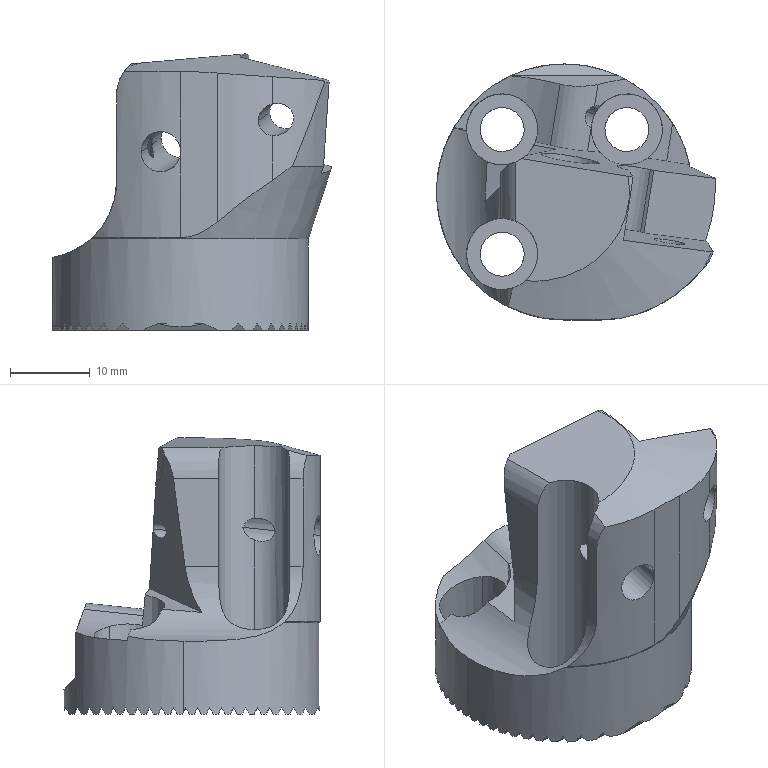NC program | Mastercam | posted with a generic post
Lines 6703 to 7888 of 7888:
(12 FEMR |TOOL - 4|DIA. OFF. - 4|LEN. - 4|TOOL DIA. - 12.)
N3534 T4 M6
N3536 G0 G54 G90 X-14.045 Y10.129 C-102.311 B-16.13 S3500 M3
N3538 G43 H4 Z65.102
N3540 Z17.102
N3542 G1 Z15.352 F2000.
N3544 X-12.727 Y9.028 Z15.201
N3546 G3 X-11.738 Y8.504 Z15.102 I1.732 J2.072
N3548 G1 X-11.151 Y8.336
N3550 X-11.015 Y8.564
N3552 G3 X-10.442 Y10.028 I-12.999 J5.944
N3554 G2 X-7.242 Y13.686 I6.178 J-2.175
N3556 X-3.552 Y14.596 I3.801 J-7.478
N3558 X-.802 Y14.328 I.15 J-12.665
N3560 X-.481 Y14.256 I-2.599 J-12.397
N3562 X1.84 Y13.588 I-5.294 J-22.736
N3564 G1 X1.993 Y13.964
N3566 X2.147 Y14.341
N3568 G3 X2.287 Y14.803 Z15.134 I-2.502 J1.016
N3570 X1.079 Y17.644 Z15.352 I-2.643 J.554
N3572 X.198 Y17.999 I-1.435 J-2.287
N3574 X-1.363 Y17.862 I-.554 J-2.643
N3576 G1 X-11.97 Y13.595 F9500.
N3578 G3 X-13.605 Y11.644 I1.007 J-2.505
N3580 X-13.648 Y11.37 I2.643 J-.554
N3582 X-11.704 Y8.494 Z15.102 I2.686 J-.28 F2000.
N3584 G1 X-11.118 Y8.327
N3586 X-11.094 Y8.32
N3588 G3 X-10.684 Y8.999 I-2.593 J2.03
N3590 G2 X-5.541 Y13.373 I7.474 J-3.577
N3592 X-1.371 Y13.742 I3.019 J-10.401
N3594 X.451 Y13.496 I-4.751 J-42.131
N3596 X1.721 Y13.293 I-1.718 J-14.847
N3598 G1 X1.874 Y13.67
N3600 X2.027 Y14.047
N3602 G3 X2.168 Y14.509 Z15.134 I-2.502 J1.016
N3604 X.96 Y17.35 Z15.352 I-2.643 J.554
N3606 X.08 Y17.705 I-1.435 J-2.287 F9500.
N3608 X-1.44 Y17.585 I-.554 J-2.643
N3610 G1 X-11.864 Y13.594
N3612 G3 X-13.542 Y11.626 I.965 J-2.522
N3614 X-13.584 Y11.352 I2.643 J-.554
N3616 X-11.641 Y8.476 Z15.102 I2.685 J-.28 F2000.
N3618 G1 X-11.054 Y8.308
N3620 X-11.022 Y8.299
N3622 G3 X-10.735 Y8.651 I-1.313 J1.369
N3624 G2 X-8.574 Y10.989 I9.204 J-6.338
N3626 X-3.748 Y13.028 I6.128 J-7.774
N3628 X-.057 Y13.105 I2.194 J-16.712
N3630 G3 X1.169 Y13.049 I2.21 J34.681
N3632 G2 X1.606 Y13.011 I-.779 J-11.644
N3634 G1 X1.759 Y13.388
N3636 X1.913 Y13.765
N3638 G3 X2.053 Y14.227 Z15.134 I-2.501 J1.016
N3640 X.846 Y17.068 Z15.352 I-2.642 J.554
N3642 X-.035 Y17.423 I-1.435 J-2.286 F9500.
N3644 X-1.515 Y17.317 I-.554 J-2.642
N3646 G1 X-11.737 Y13.583
N3648 G3 X-13.453 Y11.601 I.927 J-2.536
N3650 X-13.496 Y11.327 I2.643 J-.554
N3652 X-11.553 Y8.451 Z15.102 I2.686 J-.28 F2000.
N3654 G1 X-10.966 Y8.283
N3656 X-10.911 Y8.268
N3658 G3 X-10.36 Y8.798 I-2.825 J3.488
N3660 G2 X-7.106 Y11.303 I8.864 J-8.152
N3662 X-2.798 Y12.561 I5.527 J-10.906
N3664 X.131 Y12.699 I2.704 J-26.227
N3666 G3 X.733 Y12.722 I-.134 J11.466
N3668 G2 X1.494 Y12.735 I.545 J-10.028
N3670 G1 X1.647 Y13.112
N3672 X1.801 Y13.489
N3674 G3 X1.941 Y13.952 Z15.134 I-2.501 J1.016
N3676 X.734 Y16.793 Z15.352 I-2.642 J.554
N3678 X-.147 Y17.148 I-1.435 J-2.287 F9500.
N3680 X-1.597 Y17.053 I-.554 J-2.643
N3682 G1 X-11.552 Y13.55
N3684 G3 X-13.298 Y11.556 I.896 J-2.547
N3686 X-13.341 Y11.282 I2.643 J-.554
N3688 X-11.398 Y8.406 Z15.102 I2.686 J-.28 F2000.
N3690 G1 X-10.81 Y8.239
N3692 X-10.731 Y8.216
N3694 G3 X-10.082 Y8.726 I-2.872 J4.324
N3696 G2 X-6.668 Y10.949 I9.276 J-10.51
N3698 X-2.761 Y12.063 I5.886 J-13.243
N3700 X.33 Y12.36 I5.444 J-40.371
N3702 X1.387 Y12.471 I2.596 J-19.798
N3704 G1 X1.54 Y12.847
N3706 X1.693 Y13.225
N3708 G3 X1.835 Y13.687 Z15.134 I-2.502 J1.016
N3710 X.626 Y16.527 Z15.352 I-2.643 J.554
N3712 X-.254 Y16.883 I-1.435 J-2.286 F9500.
N3714 X-1.681 Y16.795 I-.554 J-2.642
N3716 G1 X-11.329 Y13.501
N3718 G3 X-13.099 Y11.499 I.872 J-2.555
N3720 X-13.142 Y11.225 I2.643 J-.554
N3722 X-11.199 Y8.35 Z15.102 I2.686 J-.28 F2000.
N3724 G1 X-10.612 Y8.182
N3726 X-10.515 Y8.155
N3728 G3 X-9.836 Y8.598 I-2.432 J4.464
N3730 G2 X-6.087 Y10.689 I10.05 J-13.614
N3732 X-1.813 Y11.757 I6.66 J-17.566
N3734 X.191 Y12.025 I17.327 J-122.508
N3736 G3 X.868 Y12.143 I-2.05 J13.62
N3738 G1 X1.278 Y12.202
N3740 X1.584 Y12.956
N3742 G3 X1.725 Y13.419 Z15.134 I-2.502 J1.016
N3744 X.517 Y16.26 Z15.352 I-2.643 J.554
N3746 X-.364 Y16.615 I-1.435 J-2.287 F9500.
N3748 X-1.768 Y16.535 I-.554 J-2.643
N3750 G1 X-11.083 Y13.444
N3752 G3 X-12.874 Y11.436 I.85 J-2.562
N3754 X-12.918 Y11.161 I2.642 J-.554
N3756 X-10.974 Y8.286 Z15.102 I2.686 J-.279 F2000.
N3758 G1 X-10.387 Y8.118
N3760 X-10.278 Y8.087
N3762 G3 X-9.187 Y8.705 I-3.238 J6.975
N3764 G2 X-2.697 Y11.196 I10.074 J-16.552
N3766 X.138 Y11.709 I19.12 J-97.624
N3768 G3 X.723 Y11.844 I-1.652 J8.429
N3770 X1.246 Y12.124 I-.287 J1.166
N3772 G1 X1.4 Y12.502
N3774 G3 X1.541 Y12.964 Z15.134 I-2.502 J1.016
N3776 X.333 Y15.805 Z15.352 I-2.643 J.554
N3778 X-.548 Y16.16 I-1.435 J-2.287 F9500.
N3780 X-1.888 Y16.101 I-.554 J-2.643
N3782 G1 X-10.777 Y13.396
N3784 G3 X-12.632 Y11.367 I.787 J-2.582
N3786 X-12.676 Y11.092 I2.642 J-.554
N3788 X-10.732 Y8.217 Z15.102 I2.686 J-.279 F2000.
N3790 G1 X-10.145 Y8.049
N3792 X-10.024 Y8.014
N3794 G3 X-8.95 Y8.531 I-2.555 J6.683
N3796 G2 X-2.37 Y10.876 I11.451 J-21.727
N3798 X-1.139 Y11.137 I24.943 J-114.966
N3800 G3 X.619 Y11.598 I-2.308 J12.36
N3802 X1.181 Y11.965 I-.348 J1.149
N3804 X.196 Y12.389 Z15.174 I-1.539 J-2.218
N3806 X-.074 Y12.432 Z15.192 I-.554 J-2.643
N3808 G1 X-2.477 Y12.686 Z15.352
N3810 X-9.452 Y13.425 F9500.
N3812 G3 X-12.379 Y11.294 I-.284 J-2.685
N3814 X-12.422 Y11.02 I2.642 J-.554
N3816 X-10.479 Y8.144 Z15.102 I2.686 J-.28 F2000.
N3818 G1 X-9.892 Y7.976
N3820 X-9.759 Y7.939
N3822 G3 X-8.715 Y8.363 I-2. J6.404
N3824 G2 X-2.071 Y10.586 I13.739 J-30.031
N3826 G3 X.096 Y11.184 I-5.217 J23.133
N3828 G2 X.571 Y11.365 I4.088 J-10.083
N3830 G3 X1.081 Y11.716 I-.405 J1.129
N3832 X.102 Y12.136 Z15.173 I-1.533 J-2.223
N3834 X-.104 Y12.171 Z15.187 I-.554 J-2.643
N3836 G1 X-2.572 Y12.492 Z15.352
N3838 X-9.127 Y13.343 F9500.
N3840 G3 X-12.118 Y11.219 I-.348 J-2.678
N3842 X-12.16 Y10.945 I2.643 J-.554
N3844 X-10.217 Y8.069 Z15.102 I2.685 J-.28 F2000.
N3846 G1 X-9.63 Y7.901
N3848 X-9.486 Y7.861
N3850 G3 X-8.479 Y8.205 I-1.558 J6.194
N3852 G2 X-2.184 Y10.226 I18.295 J-46.178
N3854 G3 X-.029 Y10.893 I-5.648 J22.07
N3856 X.464 Y11.105 I-6.328 J15.409
N3858 X1.096 Y11.753 I-.481 J1.099
N3860 X1.237 Y12.215 Z15.134 I-2.502 J1.016
N3862 X.029 Y15.056 Z15.352 I-2.643 J.554
N3864 X-.852 Y15.412 I-1.435 J-2.287 F9500.
N3866 X-2.133 Y15.37 I-.554 J-2.643
N3868 G1 X-9.933 Y13.189
N3870 G3 X-11.849 Y11.142 I.727 J-2.6
N3872 X-11.891 Y10.868 I2.643 J-.554
N3874 X-9.948 Y7.992 Z15.102 I2.685 J-.28 F2000.
N3876 G1 X-9.361 Y7.825
N3878 X-9.206 Y7.781
N3880 G3 X-7.874 Y8.175 I-2.845 J12.051
N3882 G1 X-7.495 Y8.301
N3884 G2 X-2.261 Y9.89 I31.197 J-93.314
N3886 G3 X-.166 Y10.599 I-5.352 J19.291
N3888 X.409 Y10.873 I-4.201 J9.531
N3890 X.992 Y11.498 I-.528 J1.077
N3892 X1.133 Y11.96 Z15.134 I-2.502 J1.016
N3894 X-.075 Y14.801 Z15.352 I-2.643 J.554
N3896 X-.955 Y15.157 I-1.435 J-2.287 F9500.
N3898 X-2.214 Y15.121 I-.554 J-2.643
N3900 G1 X-9.636 Y13.117
N3902 G3 X-11.574 Y11.064 I.704 J-2.607
N3904 X-11.617 Y10.79 I2.643 J-.554
N3906 X-9.674 Y7.914 Z15.102 I2.686 J-.28 F2000.
N3908 G1 X-9.087 Y7.746
N3910 X-8.92 Y7.699
N3912 G3 X-7.646 Y8.009 I-2.004 J10.96
N3914 X-4.554 Y8.914 I-96.959 J337.459
N3916 G1 X-4.161 Y9.027
N3918 G3 X-1.041 Y10. I-13.289 J48.096
N3920 X.364 Y10.645 I-2.859 J8.087
N3922 X.826 Y11.09 I-.571 J1.056
N3924 X.135 Y11.337 Z15.151 I-1.248 J-2.395
N3926 G1 X-2.833 Y11.963 Z15.352
N3928 X-8.096 Y13.072 F9500.
N3930 X-8.099 Y13.073
N3932 G3 X-11.295 Y10.984 I-.554 J-2.643
N3934 X-11.338 Y10.71 I2.643 J-.554
N3936 X-9.394 Y7.834 Z15.102 I2.685 J-.28 F2000.
N3938 G1 X-8.807 Y7.667
N3940 X-8.627 Y7.615
N3942 G3 X-7.07 Y7.937 I-1.611 J11.688
N3944 X-1.999 Y9.39 I-21.287 J83.884
N3946 X.024 Y10.243 I-3.535 J11.216
N3948 G1 X.31 Y10.413
N3950 G3 X.706 Y10.796 I-.612 J1.032
N3952 G1 X.86 Y11.172
N3954 G3 X1.001 Y11.634 Z15.134 I-2.502 J1.016
N3956 X-.207 Y14.476 Z15.352 I-2.643 J.554
N3958 X-1.088 Y14.831 I-1.435 J-2.287 F9500.
N3960 X-2.354 Y14.793 I-.554 J-2.643
N3962 G1 X-9.08 Y12.954
N3964 G3 X-11.011 Y10.903 I.712 J-2.604
N3966 X-11.054 Y10.629 I2.643 J-.554
N3968 X-9.11 Y7.753 Z15.102 I2.686 J-.28 F2000.
N3970 G1 X-8.523 Y7.585
N3972 X-8.328 Y7.53
N3974 G3 X-6.513 Y7.847 I-1.451 J13.642
N3976 X-3.182 Y8.74 I-10.173 J44.586
N3978 G1 X-2.808 Y8.899
N3980 X-.039 Y10.075
N3982 G3 X.523 Y10.484 I-.773 J1.658
N3984 X.691 Y10.758 I-.843 J.704
N3986 X.832 Y11.22 Z15.134 I-2.501 J1.016
N3988 X.889 Y11.698 Z15.166 I-2.642 J.554
N3990 G1 X.902 Y12.181 Z15.198
N3992 G3 X.022 Y14.253 Z15.352 I-2.699 J.075
N3994 X-1.242 Y14.899 I-1.818 J-1.996 F9500.
N3996 X-4.439 Y12.81 I-.554 J-2.643
N3998 X-4.063 Y10.79 I2.643 J-.554
N4000 X-2.35 Y9.614 Z15.211 I2.267 J1.466 F2000.
N4002 X-.746 Y9.77 Z15.102 I.554 J2.642
N4004 G1 X-.184 Y10.007
N4006 G3 X.387 Y10.323 I-.445 J1.48
N4008 X.691 Y10.758 I-.807 J.887
N4010 G1 X.845 Y11.135
N4012 G3 X.986 Y11.597 Z15.134 I-2.502 J1.016
N4014 X-.222 Y14.439 Z15.352 I-2.643 J.554
N4016 X-1.103 Y14.794 I-1.435 J-2.287 F9500.
N4018 X-2.418 Y14.742 I-.554 J-2.643
N4020 G1 X-8.84 Y12.857
N4022 G3 X-10.722 Y10.82 I.761 J-2.591
N4024 X-10.765 Y10.546 I2.643 J-.554
N4026 X-8.822 Y7.67 Z15.102 I2.686 J-.28 F2000.
N4028 G1 X-8.235 Y7.503
N4030 X-8.024 Y7.443
N4032 G3 X-6.305 Y7.678 I-.718 J11.658
N4034 X-5.129 Y7.936 I-5.598 J28.259
N4036 X-4.566 Y8.156 I-.661 J2.523
N4038 G1 X-4.19 Y8.315
N4040 X-2.691 Y8.948
N4042 G3 X-1.099 Y10.881 Z15.275 I-1.051 J2.487
N4044 X-1.11 Y12.038 Z15.352 I-2.642 J.554
N4046 X-3.187 Y14.077 I-2.632 J-.603 F9500.
N4048 X-4.54 Y14.015 I-.554 J-2.642
N4050 G1 X-8.586 Y12.762
N4052 G3 X-10.429 Y10.737 I.799 J-2.579
N4054 X-10.473 Y10.463 I2.642 J-.554
N4056 X-8.529 Y7.587 Z15.102 I2.686 J-.279 F2000.
N4058 G1 X-7.942 Y7.419
N4060 X-7.712 Y7.354
N4062 G3 X-6.217 Y7.497 I-.189 J9.798
N4064 X-5.935 Y7.578 I-.186 J1.186
N4066 G1 X-5.56 Y7.736
N4068 X-4.436 Y8.211
N4070 G3 X-2.844 Y10.144 Z15.275 I-1.051 J2.488
N4072 X-2.854 Y11.301 Z15.352 I-2.643 J.554
N4074 X-4.932 Y13.342 I-2.633 J-.603 F9500.
N4076 X-6.26 Y13.285 I-.554 J-2.643
N4078 G1 X-8.265 Y12.685
N4080 G3 X-10.133 Y10.653 I.774 J-2.586
N4082 X-10.177 Y10.378 I2.642 J-.554
N4084 X-8.233 Y7.503 Z15.102 I2.686 J-.279 F2000.
N4086 G1 X-7.646 Y7.335
N4088 X-7.391 Y7.262
N4090 G3 X-6.836 Y7.271 I.198 J4.739
N4092 X-6.442 Y7.364 I-.073 J1.197
N4094 G1 X-6.067 Y7.522
N4096 X-5.317 Y7.839
N4098 G3 X-3.725 Y9.772 Z15.275 I-1.05 J2.487
N4100 X-3.736 Y10.929 Z15.352 I-2.642 J.554
N4102 X-5.814 Y12.969 I-2.632 J-.603 F9500.
N4104 X-7.335 Y12.846 I-.554 J-2.642
N4106 G1 X-8.154 Y12.532
N4108 G3 X-9.829 Y10.566 I.967 J-2.52
N4110 X-9.872 Y10.292 I2.642 J-.554
N4112 X-7.928 Y7.416 Z15.102 I2.686 J-.28 F2000.
N4114 X-7.342 Y7.249 I5.983 J19.895
N4116 X-7.292 Y7.237 I.296 J1.163
N4118 X-6.579 Y7.305 I.246 J1.175
N4120 G1 X-6.204 Y7.464
N4122 X-5.829 Y7.623
N4124 G3 X-4.91 Y8.262 Z15.201 I-1.051 J2.488
N4126 G1 X-3.736 Y9.515 Z15.352
N4128 G0 Z65.102
N4130 M5
N4132 G0 G28 G91 Z0.
N4134 G28 C0. B0.
N4136 M01
N4138 G0 G17 G40 G80 G90 G94 G98
N4140 G0 G28 G91 Z0.
(12 FEMF |TOOL - 9|DIA. OFF. - 9|LEN. - 9|TOOL DIA. - 12.)
N4142 T9 M6
N4144 G0 G54 G90 X-12.135 Y4.85 C-102.311 B-16.13 S3500 M3
N4146 G43 H9 Z66.002
N4148 Z17.002
N4150 G1 Z15.002 F2000.
N4152 G41 D9 X-8.911 Y6.212 F600.
N4154 X2.871 Y11.189
N4156 G40 X8.398 Y13.523
N4158 G0 Z66.002
N4160 M5
N4162 G0 G28 G91 Z0.
N4164 G28 C0. B0.
N4166 M01
N4168 G0 G17 G40 G80 G90 G94 G98
N4170 G0 G28 G91 Z0.
(2.5 BM |TOOL - 15|DIA. OFF. - 15|LEN. - 15|TOOL DIA. - 2.5)
N4172 T15 M6
N4174 G0 G54 G90 X20.642 Y15.943 C46.126 B-90. S4500 M3
N4176 G43 H15 Z47.39
N4178 Y12.068
N4180 Z35.871
N4182 Z17.871
N4184 G1 Z15.871 F600.
N4186 X20.661 Z15.456 F1000.
N4188 X20.709 Z15.043
N4190 X20.706 Y12.063 Z14.97
N4192 X20.681 Y12.051 Z14.901
N4194 X20.637 Y12.032 Z14.838
N4196 X20.579 Y12.008 Z14.781
N4198 X20.437 Y11.953 Z14.693
N4200 X20.288 Y11.897 Z14.649
N4202 X19.569 Y11.528 Z14.635 C46.54
N4204 X18.849 Y11.159 Z14.616 C46.954
N4206 X18.129 Y10.792 Z14.593 C47.368
N4208 X17.397 Y10.395 Z14.566 C47.793
N4210 X16.662 Y10.019 Z14.531 C48.217
N4212 X15.928 Y9.533 Z14.552 C49.01
N4214 X15.193 Y9.052 Z14.565 C49.818
N4216 X14.539 Y8.609 Z14.567 C50.545
N4218 X13.884 Y8.18 Z14.56 C51.27
N4220 X13.229 Y7.743 Z14.543 C51.996
N4222 X12.576 Y7.316 Z14.512 C52.673
N4224 X11.916 Y6.899 Z14.47 C53.354
N4226 X11.585 Y6.689 Z14.455 C53.695
N4228 X11.419 Y6.584 Z14.447 C53.865
N4230 X11.336 Y6.532 Z14.443 C53.951
N4232 X11.253 Y6.485 Z14.437 C54.017
N4234 X11.185 Y6.464 Z14.446 C54.068
N4236 X11.117 Y6.443 Z14.455 C54.119
N4238 X11.049 Y6.422 Z14.464 C54.17
N4240 X10.981 Y6.401 Z14.473 C54.222
N4242 X10.844 Y6.358 Z14.491 C54.325
N4244 X10.707 Y6.315 Z14.515 C54.428
N4246 X9.934 Y6.092 Z14.606 C54.947
N4248 X9.899 Y6.073 Z14.611 C54.972
N4250 X9.894 Y6.061 Z14.612 C54.979
N4252 X9.889 Y6.047 C54.988
N4254 X9.884 Y6.034 Z14.613 C54.995
N4256 X9.881 Y6.019 Z14.614 C55.004
N4258 X9.89 Y6.018 Z14.613 C55.011
N4260 X9.899 Y6.017 Z14.612 C55.017
N4262 X9.909 Y6.016 Z14.609 C55.024
N4264 X9.918 Y6.015 Z14.606 C55.031
N4266 X9.929 Z14.604 C55.038
N4268 X9.926 Y5.999 Z14.603 C55.048
N4270 Y5.981 Z14.602 C55.058
N4272 X9.922 Y5.959 Z14.601 C55.07
N4274 X9.926 Y5.933 Z14.598 C55.085
N4276 X9.93 Y5.907 Z14.594 C55.101
N4278 X9.934 Y5.881 Z14.591 C55.116
N4280 X9.938 Y5.855 Z14.587 C55.131
N4282 X9.941 Y5.828 Z14.582 C55.147
N4284 X9.944 Y5.801 Z14.578 C55.163
N4286 X9.947 Y5.774 Z14.574 C55.179
N4288 X9.95 Y5.746 Z14.57 C55.195
N4290 X9.954 Y5.717 Z14.568 C55.211
N4292 X9.958 Y5.689 Z14.567 C55.228
N4294 X9.964 Y5.66 Z14.568 C55.244
N4296 Y5.651 Z14.571 C55.25
N4298 X10.017 Y5.103 Z14.744 C55.572
N4300 X10.046 Y4.758 Z14.849 C55.717
N4302 X10.074 Y4.417 Z14.945 C55.859
N4304 X10.102 Y4.093 Z15.029 C55.934
N4306 X10.13 Y3.768 Z15.107 C56.008
N4308 X10.157 Y3.45 Z15.176 C56.051
N4310 X10.184 Y3.13 Z15.239 C56.095
N4312 X10.211 Y2.837 Z15.291 C56.044
N4314 X10.238 Y2.543 Z15.338 C55.993
N4316 X10.263 Y2.275 Z15.376 C55.849
N4318 X10.29 Y2.006 Z15.41 C55.705
N4320 X10.315 Y1.754 Z15.438 C55.502
N4322 X10.34 Y1.502 Z15.461 C55.3
N4324 X10.365 Y1.266 Z15.48 C55.039
N4326 X10.396 Y.945 Z15.503 C54.685
N4328 X10.414 Y.776 Z15.514 C54.387
N4330 X10.433 Y.605 Z15.525 C54.087
N4332 X10.464 Y.354 Z15.538 C53.645
N4334 X10.487 Y.221 Z15.539 C53.337
N4336 X10.518 Y.04 Z15.542 C52.914
N4338 X10.545 Y-.114 Z15.552 C52.372
N4340 X10.582 Y-.266 Z15.551 C51.836
N4342 X10.62 Y-.396 Z15.55 C51.259
N4344 X10.644 Y-.484 Z15.554 C50.87
N4346 X10.674 Y-.572 Z15.55 C50.477
N4348 X10.704 Y-.661 Z15.548 C50.08
N4350 X10.757 Y-.788 Z15.549 C49.286
N4352 X10.801 Y-.86 Z15.545 C48.692
N4354 X10.844 Y-.932 Z15.542 C48.1
N4356 X10.889 Y-.988 C47.462
N4358 X10.912 Y-1.014 Z15.539 C47.161
N4360 X10.974 Y-1.082 Z15.534 C46.386
N4362 X11.034 Y-1.151 Z15.536 C45.595
N4364 X11.109 Y-1.196 Z15.531 C44.689
N4366 X11.179 Y-1.242 Z15.533 C43.8
N4368 X11.269 Y-1.262 Z15.528 C42.742
N4370 X11.342 Y-1.278 C41.882
N4372 X11.447 Y-1.299 C40.716
N4374 X11.518 Y-1.312 Z15.531 C39.935
N4376 X11.567 Y-1.311 Z15.533 C39.384
N4378 X11.64 Y-1.307 C38.619
N4380 X11.715 Y-1.294 Z15.534 C37.821
N4382 X11.778 Y-1.282 Z15.536 C37.175
N4384 X11.855 Y-1.267 Z15.537 C36.402
N4386 X11.935 Y-1.251 Z15.538 C35.63
N4388 X12.005 Y-1.237 Z15.539 C34.973
N4390 X12.079 Y-1.221 Z15.54 C34.296
N4392 X12.158 Y-1.203 Z15.538 C33.619
N4394 X12.177 Y-1.194 Z15.537 C33.474
N4396 X12.197 Y-1.185 Z15.534 C33.329
N4398 X12.217 Y-1.175 Z15.528 C33.185
N4400 X12.236 Y-1.164 Z15.519 C33.041
N4402 X12.256 Y-1.151 Z15.509 C32.893
N4404 X12.275 Y-1.138 Z15.496 C32.746
N4406 X12.294 Y-1.123 Z15.481 C32.599
N4408 X12.312 Y-1.107 Z15.464 C32.453
N4410 X12.33 Y-1.091 Z15.445 C32.308
N4412 X12.348 Y-1.073 Z15.425 C32.164
N4414 X12.365 Y-1.054 Z15.403 C32.021
N4416 X12.381 Y-1.034 Z15.38 C31.878
N4418 X12.464 Y-.945 Z15.258 C31.001
N4420 X12.684 Y-.73 Z14.958 C28.836
N4422 X12.926 Y-.525 Z14.656 C26.6
N4424 X13.195 Y-.306 Z14.354 C24.182
N4426 X13.472 Y-.106 Z14.067 C21.862
N4428 X13.765 Y.098 Z13.789 C19.483
N4430 X14.154 Y.338 Z13.449 C16.479
N4432 X14.253 Y.396 Z13.367 C15.605
N4434 X14.335 Y.442 Z13.295 C14.849
N4436 X14.401 Y.48 Z13.233 C14.21
N4438 X14.482 Y.519 Z13.159 C13.34
N4440 X14.547 Y.551 Z13.096 C12.588
N4442 X14.598 Y.581 Z13.042 C11.928
N4444 X14.659 Y.614 Z12.979 C11.033
N4446 X14.706 Y.64 Z12.926 C10.257
N4448 X14.743 Y.661 Z12.88 C9.601
N4450 X14.783 Y.683 Z12.83 C8.709
N4452 X14.812 Y.7 Z12.788 C7.937
N4454 X14.833 Y.714 Z12.753 C7.284
N4456 X14.852 Y.729 Z12.716 C6.396
N4458 X14.863 Y.74 Z12.687 C5.627
N4460 X14.868 Y.753 Z12.663 C4.965
N4462 X14.866 Y.768 Z12.641 C4.063
N4464 X14.858 Y.781 Z12.624 C3.282
N4466 X14.848 Y.792 Z12.611 C2.622
N4468 X14.824 Y.808 Z12.604 C1.724
N4470 X14.798 Y.823 Z12.6 C.946
N4472 X14.773 Y.836 Z12.598 C.288
N4474 X14.728 Y.856 Z12.605 C-.608
N4476 X14.684 Y.875 Z12.613 C-1.383
N4478 X14.643 Y.884 Z12.623 C-2.002
N4480 X14.579 Y.9 Z12.644 C-2.847
N4482 X14.517 Y.909 Z12.665 C-3.546
N4484 X14.461 Y.92 Z12.685 C-4.137
N4486 X14.377 Y.938 Z12.718 C-4.944
N4488 X14.299 Y.959 Z12.749 C-5.643
N4490 X14.215 Y.984 Z12.783 C-6.341
N4492 X14.14 Y1.008 Z12.814 C-6.932
N4494 X14.047 Y1.042 Z12.853 C-7.63
N4496 X13.778 Y1.152 Z12.97 C-9.515
N4498 X13.615 Y1.222 Z13.045 C-10.674
N4500 X13.457 Y1.292 Z13.122 C-11.832
N4502 X13.303 Y1.354 Z13.202 C-12.956
N4504 X13.153 Y1.416 Z13.285 C-14.081
N4506 X13.007 Y1.479 Z13.37 C-15.205
N4508 X12.866 Y1.543 Z13.456 C-16.33
N4510 X12.729 Y1.608 Z13.546 C-17.454
N4512 X12.596 Y1.673 Z13.637 C-18.579
N4514 X12.468 Y1.74 Z13.732 C-19.703
N4516 X12.345 Y1.808 Z13.828 C-20.828
N4518 X12.225 Y1.879 Z13.927 C-21.953
N4520 X12.111 Y1.951 Z14.028 C-23.079
N4522 X12.001 Y1.968 Z14.14 C-23.992
N4524 X11.895 Y1.987 Z14.253 C-24.905
N4526 X11.794 Y2.007 Z14.37 C-25.819
N4528 X11.699 Y2.029 Z14.488 C-26.733
N4530 X11.607 Y2.053 Z14.61 C-27.648
N4532 X11.521 Y2.078 Z14.734 C-28.562
N4534 X11.435 Y2.108 Z14.867 C-29.518
N4536 X11.364 Y2.135 Z14.985 C-30.372
N4538 X11.218 Y2.208 Z15.262 C-32.276
N4540 X11.202 Y2.215 Z15.276 C-32.378
N4542 X11.186 Y2.223 Z15.289 C-32.481
N4544 X11.173 Y2.23 Z15.305 C-32.584
N4546 X11.159 Y2.237 Z15.32 C-32.689
N4548 X11.144 Y2.244 Z15.335 C-32.796
N4550 X11.128 Y2.252 Z15.349 C-32.905
N4552 X11.111 Y2.259 Z15.363 C-33.018
N4554 X11.092 Y2.266 Z15.377 C-33.133
N4556 X11.073 Y2.274 Z15.39 C-33.252
N4558 X11.053 Y2.281 Z15.403 C-33.374
N4560 X11.035 Y2.289 Z15.419 C-33.502
N4562 X10.953 Y2.27 Z15.42 C-34.696
N4564 X10.901 Y2.258 Z15.424 C-35.443
N4566 X10.853 Y2.242 Z15.421 C-36.294
N4568 X10.801 Y2.228 Z15.425 C-37.114
N4570 X10.736 Y2.202 Z15.42 C-38.383
N4572 X10.684 Y2.159 Z15.429 C-39.249
N4574 X10.631 Y2.107 Z15.431 C-40.271
N4576 X10.595 Y2.068 Z15.434 C-41.017
N4578 X10.552 Y2.02 Z15.438 C-41.939
N4580 X10.517 Y1.975 Z15.439 C-42.781
N4582 X10.483 Y1.93 Z15.442 C-43.63
N4584 X10.45 Y1.884 Z15.446 C-44.48
N4586 X10.419 Y1.833 Z15.445 C-45.425
N4588 X10.391 Y1.783 C-46.336
N4590 X10.363 Y1.738 Z15.451 C-47.181
N4592 X10.339 Y1.689 Z15.45 C-48.08
N4594 X10.315 Y1.642 Z15.453 C-48.968
N4596 X10.293 Y1.594 Z15.456 C-49.854
N4598 X10.274 Y1.537 Z15.451 C-50.892
N4600 X10.257 Y1.495 Z15.454 C-51.661
N4602 X10.239 Y1.451 Z15.456 C-52.485
N4604 X10.222 Y1.408 Z15.461 C-53.279
N4606 X10.206 Y1.352 Z15.457 C-54.298
N4608 X10.192 Y1.303 C-55.191
N4610 X10.179 Y1.258 Z15.458 C-56.014
N4612 X10.166 Y1.213 Z15.459 C-56.836
N4614 X10.151 Y1.206 Z15.455 C-58.036
N4616 X10.137 Y1.2 Z15.453 C-59.083
N4618 X10.125 Y1.195 Z15.451 C-60.084
N4620 X10.114 Y1.191 Z15.452 C-60.856
N4622 X10.113 Z15.454 C-60.91
N4624 Y1.192 Z15.46 C-60.966
N4626 Y1.194 Z15.468 C-61.023
N4628 X10.111 Y1.198 Z15.477 C-61.079
N4630 X10.108 Y1.202 Z15.487 C-61.135
N4632 X10.103 Y1.207 Z15.497 C-61.189
N4634 X10.097 Y1.213 Z15.507 C-61.244
N4636 X10.09 Y1.219 Z15.517 C-61.297
N4638 X10.083 Y1.226 Z15.526 C-61.349
N4640 X10.075 Y1.233 Z15.535 C-61.4
N4642 X10.066 Y1.241 Z15.544 C-61.449
N4644 X10.057 Y1.248 Z15.552 C-61.497
N4646 X10.048 Y1.255 Z15.56 C-61.544
N4648 X10.041 Y1.264 Z15.568 C-61.589
N4650 X10.037 Y1.267 Z15.576 C-61.632
N4652 X10.033 Y1.271 Z15.584 C-61.675
N4654 X10.028 Y1.276 Z15.592 C-61.723
N4656 X10.024 Y1.28 Z15.6 C-61.77
N4658 X10.023 Y1.283 Z15.609 C-61.83
N4660 X10.021 Y1.286 Z15.617 C-61.889
N4662 X10.025 Y1.289 Z15.627 C-61.97
N4664 X10.028 Y1.292 Z15.636 C-62.051
N4666 X10.027 Y1.293 Z15.64 C-62.075
N4668 X10.025 Y1.295 Z15.644 C-62.1
N4670 X10.09 Y1.325 Z15.657 C-62.403
N4672 X10.119 Y1.337 Z15.659 C-62.536
N4674 X10.146 Y1.349 Z15.661 C-62.669
N4676 X10.173 Y1.359 Z15.662 C-62.802
N4678 X10.198 Y1.368 Z15.664 C-62.936
N4680 X10.222 Y1.376 Z15.665 C-63.07
N4682 X10.245 Y1.383 Z15.666 C-63.204
N4684 X10.266 Y1.389 Z15.667 C-63.339
N4686 X10.286 Y1.394 C-63.474
N4688 X10.304 Y1.398 Z15.668 C-63.609
N4690 X10.321 Y1.401 C-63.744
N4692 X10.336 Y1.404 C-63.88
N4694 X10.35 Y1.406 C-64.017
N4696 X10.362 Y1.407 C-64.155
N4698 X10.372 Y1.406 Z15.667 C-64.288
N4700 X10.38 Y1.405 Z15.666 C-64.422
N4702 X10.386 Y1.404 Z15.665 C-64.557
N4704 X10.39 Y1.402 Z15.664 C-64.693
N4706 X10.392 Y1.4 Z15.662 C-64.829
N4708 Y1.395 Z15.66 C-64.957
N4710 X10.39 Y1.39 Z15.657 C-65.085
N4712 X10.318 Y1.358 Z15.663 C-66.198
N4714 X10.279 Y1.318 Z15.652 C-67.149
N4716 X10.236 Y1.281 Z15.651 C-68.061
N4718 X10.191 Y1.239 Z15.649 C-69.07
N4720 X10.16 Y1.205 Z15.648 C-69.883
N4722 X10.126 Y1.166 Z15.646 C-70.791
N4724 X10.096 Y1.127 Z15.645 C-71.702
N4726 X10.08 Y1.095 Z15.638 C-72.435
N4728 X10.043 Y1.049 Z15.643 C-73.519
N4730 X10.021 Y1.009 Z15.641 C-74.432
N4732 X10.001 Y.969 Z15.64 C-75.345
N4734 X9.977 Y.918 Z15.639 C-76.502
N4736 X9.967 Y.877 Z15.637 C-77.135
N4738 X9.955 Y.819 Z15.634 C-78.026
N4740 X9.939 Y.765 Z15.637 C-78.854
N4742 X9.927 Y.709 C-79.717
N4744 X9.916 Y.654 Z15.638 C-80.578
N4746 X9.907 Y.603 C-81.351
N4748 X9.899 Y.553 Z15.639 C-82.122
N4750 X9.896 Y.482 Z15.633 C-83.207
N4752 X9.887 Y.421 Z15.637 C-84.053
N4754 X9.881 Y.362 Z15.638 C-84.862
N4756 X9.875 Y.3 Z15.64 C-85.709
N4758 X9.873 Y.236 Z15.639 C-86.595
N4760 X9.871 Y.174 Z15.638 C-87.442
N4762 X9.869 Y.115 Z15.639 C-88.251
N4764 X9.868 Y.053 Z15.638 C-89.099
N4766 X9.869 Y-.01 Z15.637 C-89.94
N4768 X9.87 Y-.074 Z15.636 C-90.782
N4770 X9.872 Y-.137 Z15.635 C-91.623
N4772 X9.874 Y-.201 C-92.466
N4774 X9.877 Y-.265 Z15.634 C-93.308
N4776 X9.88 Y-.328 Z15.633 C-94.148
N4778 X9.884 Y-.392 C-94.99
N4780 X9.89 Y-.444 C-95.867
N4782 X9.896 Y-.497 C-96.746
N4784 X9.902 Y-.549 C-97.623
N4786 X9.908 Y-.607 Z15.637 C-98.592
N4788 X9.917 Y-.654 Z15.636 C-99.379
N4790 X9.929 Y-.706 Z15.635 C-100.253
N4792 X9.941 Y-.758 C-101.129
N4794 X9.954 Y-.833 Z15.633 C-101.925
N4796 X9.97 Y-.908 Z15.632 C-102.722
N4798 X9.981 Y-.963 C-103.304
N4800 X10.001 Y-1.06 Z15.634 C-104.343
N4802 X10.025 Y-1.132 Z15.629 C-105.11
N4804 X10.043 Y-1.209 Z15.632 C-105.936
N4806 X10.075 Y-1.3 Z15.629 C-106.909
N4808 X10.1 Y-1.387 Z15.621 C-107.383
N4810 X10.131 Y-1.506 Z15.614 C-108.021
N4812 X10.165 Y-1.624 Z15.607 C-108.66
N4814 X10.191 Y-1.734 Z15.606 C-109.249
N4816 X10.236 Y-1.871 Z15.596 C-109.933
N4818 X10.279 Y-1.995 Z15.586 C-110.552
N4820 X10.326 Y-2.138 Z15.573 C-111.099
N4822 X10.38 Y-2.284 Z15.558 C-111.658
N4824 X10.442 Y-2.437 Z15.534 C-112.12
N4826 X10.493 Y-2.571 Z15.518 C-112.522
N4828 X10.571 Y-2.766 Z15.491 C-113.058
N4830 X10.618 Y-2.88 Z15.476 C-113.372
N4832 X10.669 Y-2.992 Z15.46 C-113.683
N4834 X10.72 Y-3.099 Z15.443 C-113.983
N4836 X10.784 Y-3.251 Z15.423 C-114.332
N4838 X10.86 Y-3.396 Z15.396 C-114.677
N4840 X10.895 Y-3.459 Z15.382 C-114.803
N4842 X10.978 Y-3.632 Z15.353 C-115.138
N4844 X11.096 Y-3.838 Z15.311 C-115.552
N4846 X11.195 Y-4.002 Z15.276 C-115.883
N4848 X11.3 Y-4.164 Z15.242 C-116.215
N4850 X11.335 Y-4.209 Z15.229 C-116.312
N4852 X11.44 Y-4.352 Z15.195 C-116.615
N4854 X11.547 Y-4.507 Z15.159 C-116.882
N4856 X11.616 Y-4.587 Z15.135 C-117.029
N4858 X11.713 Y-4.724 Z15.098 C-117.19
N4860 X11.811 Y-4.865 Z15.063 C-117.353
N4862 X11.792 Y-4.895 Z15.071 C-117.387
N4864 X11.774 Y-4.926 Z15.084 C-117.421
N4866 X11.754 Y-4.956 Z15.095 C-117.455
N4868 X11.734 Y-4.987 Z15.106 C-117.49
N4870 X11.782 Y-5.024 Z15.086 C-117.548
N4872 X11.83 Y-5.061 Z15.065 C-117.605
N4874 X11.88 Y-5.098 Z15.052 C-117.662
N4876 X11.93 Y-5.136 Z15.04 C-117.719
N4878 X11.981 Y-5.173 Z15.031 C-117.775
N4880 X12.032 Y-5.211 Z15.022 C-117.832
N4882 X12.072 Y-5.25 Z15.008 C-117.884
N4884 X12.245 Y-5.384 Z14.952 C-118.087
N4886 X12.401 Y-5.543 Z14.903 C-118.295
N4888 X12.547 Y-5.688 Z14.855 C-118.454
N4890 X12.711 Y-5.822 Z14.802 C-118.616
N4892 X12.871 Y-5.964 Z14.751 C-118.749
N4894 X13.022 Y-6.106 Z14.706 C-118.877
N4896 X13.188 Y-6.234 Z14.657 C-119.006
N4898 X13.363 Y-6.358 Z14.608 C-119.137
N4900 X13.556 Y-6.512 Z14.547 C-119.204
N4902 X13.707 Y-6.621 Z14.502 C-119.255
N4904 X13.884 Y-6.742 Z14.452 C-119.313
N4906 X14.1 Y-6.872 Z14.393 C-119.382
N4908 X14.259 Y-6.974 Z14.352 C-119.433
N4910 X14.435 Y-7.07 Z14.309 C-119.486
N4912 X14.623 Y-7.166 Z14.265 C-119.543
N4914 X14.815 Y-7.256 Z14.223 C-119.6
N4916 X14.984 Y-7.324 Z14.188 C-119.648
N4918 X15.2 Y-7.42 Z14.146 C-119.711
N4920 X15.411 Y-7.491 Z14.108 C-119.769
N4922 X15.595 Y-7.558 Z14.078 C-119.821
N4924 X15.795 Y-7.619 Z14.048 C-119.875
N4926 X16.012 Y-7.672 Z14.019 C-119.934
N4928 X16.145 Y-7.713 Z14.001 C-119.962
N4930 X16.403 Y-7.776 Z13.97 C-120.015
N4932 X16.609 Y-7.817 Z13.949 C-120.057
N4934 X16.815 Y-7.852 Z13.93 C-120.099
N4936 X17.023 Y-7.883 Z13.914 C-120.141
N4938 X17.231 Y-7.907 Z13.901 C-120.182
N4940 X17.456 Y-7.926 Z13.89 C-120.227
N4942 X17.65 Y-7.941 Z13.884 C-120.266
N4944 X17.859 Y-7.95 Z13.879 C-120.307
N4946 X18.086 Y-7.952 Z13.878 C-120.352
N4948 X18.28 Y-7.953 Z13.879 C-120.39
N4950 X18.5 Y-7.928 Z13.889 C-120.474
N4952 X19.492 Y-7.827 Z13.942 C-120.856
N4954 X20.483 Y-7.688 Z14.013 C-121.381
N4956 X21.475 Y-7.548 Z14.083 C-121.905
N4958 X22.466 Y-7.343 Z14.182 C-122.667
N4960 X23.458 Y-7.138 Z14.278 C-123.429
N4962 X24.449 Y-6.866 Z14.4 C-124.428
N4964 X25.441 Y-6.592 Z14.517 C-125.427
N4966 X26.432 Y-6.143 Z14.697 C-127.048
N4968 X27.424 Y-5.689 Z14.865 C-128.67
N4970 X28.415 Y-5.119 Z15.055 C-130.684
N4972 X29.407 Y-4.543 Z15.225 C-132.698
N4974 X29.572 Y-4.414 Z15.26 C-133.158
N4976 X29.748 Y-4.281 Z15.294 C-133.648
N4978 X29.923 Y-4.154 Z15.326 C-134.138
N4980 X30.098 Y-4.033 Z15.355 C-134.628
N4982 X30.273 Y-3.916 Z15.381 C-135.121
N4984 X30.446 Y-3.805 Z15.405 C-135.612
N4986 X30.619 Y-3.698 Z15.426 C-136.106
N4988 X30.79 Y-3.6 Z15.446 C-136.599
N4990 X31.003 Y-3.481 Z15.467 C-137.216
N4992 X31.133 Y-3.41 Z15.48 C-137.61
N4994 X31.298 Y-3.322 Z15.494 C-138.116
N4996 X31.464 Y-3.235 Z15.507 C-138.642
N4998 X31.627 Y-3.138 Z15.522 C-139.222
N5000 X31.79 Y-3.045 Z15.535 C-139.804
N5002 X31.949 Y-2.95 Z15.547 C-140.415
N5004 X32.107 Y-2.859 Z15.559 C-141.028
N5006 X32.228 Y-2.791 Z15.566 C-141.506
N5008 X32.367 Y-2.715 Z15.572 C-142.062
N5010 X32.56 Y-2.615 Z15.584 C-142.861
N5012 X32.749 Y-2.522 Z15.591 C-143.66
N5014 X32.775 Y-2.509 Z15.59 C-143.774
N5016 X32.801 Y-2.497 Z15.589 C-143.888
N5018 X32.825 Y-2.486 Z15.587 C-144.002
N5020 X32.849 Y-2.476 Z15.586 C-144.116
N5022 X32.871 Y-2.467 Z15.585 C-144.231
N5024 X32.892 Y-2.459 Z15.583 C-144.346
N5026 X32.912 Y-2.452 Z15.581 C-144.461
N5028 X32.931 Y-2.446 Z15.579 C-144.576
N5030 X32.949 Y-2.441 Z15.577 C-144.692
N5032 X32.965 Y-2.437 Z15.575 C-144.808
N5034 X32.98 Y-2.432 Z15.573 C-144.928
N5036 X32.994 Y-2.427 Z15.571 C-145.049
N5038 X33.006 Y-2.424 Z15.569 C-145.171
N5040 X33.016 Y-2.42 Z15.567 C-145.293
N5042 X33.025 Y-2.418 Z15.565 C-145.415
N5044 X33.032 Y-2.414 Z15.564 C-145.544
N5046 X33.038 Y-2.41 Z15.562 C-145.674
N5048 X33.041 Y-2.407 Z15.56 C-145.804
N5050 Y-2.386 Z15.563 C-146.706
N5052 Y-2.34 Z15.57 C-148.765
N5054 Y-2.294 Z15.576 C-150.824
N5056 Y-2.248 Z15.582 C-152.882
N5058 Y-2.225 Z15.583 C-153.793
N5060 Y-2.195 Z15.589 C-154.965
N5062 Y-2.142 Z15.596 C-157.048
N5064 Y-2.092 Z15.603 C-159.017
N5066 Y-2.051 Z15.606 C-160.582
N5068 Y-2.042 Z15.609 C-161.089
N5070 Y-2.002 Z15.613 C-163.125
N5072 Y-1.981 C-164.2
N5074 Y-1.96 Z15.618 C-165.274
N5076 Y-1.923 Z15.623 C-167.199
N5078 Y-1.901 Z15.625 C-169.176
N5080 Y-1.879 Z15.627 C-171.153
N5082 Y-1.903 Z15.625 C-172.974
N5084 X33.04 Y-1.927 Z15.627 C-174.781
N5086 X33.034 Y-1.951 Z15.645 C-176.523
N5088 X33.023 Y-1.976 Z15.68 C-178.295
N5090 X33.007 Y-2.106 Z15.72 C-179.702
N5092 X32.987 Y-2.235 Z15.777 C-181.121
N5094 X32.961 Y-2.363 Z15.852 C-182.554
N5096 X32.929 Y-2.49 Z15.945 C-184.007
N5098 X32.892 Y-2.615 Z16.056 C-185.479
N5100 X32.85 Y-2.72 Z16.194 C-187.096
N5102 X32.823 Y-2.783 Z16.281 C-188.097
N5104 X32.806 Y-2.824 Z16.337 C-188.755
N5106 X32.782 Y-2.88 Z16.415 C-189.677
N5108 X32.763 Y-2.925 Z16.478 C-190.425
N5110 X32.742 Y-2.974 Z16.547 C-191.258
N5112 X32.72 Y-3.023 Z16.617 C-192.107
N5114 X32.702 Y-3.065 Z16.676 C-192.838
N5116 X32.678 Y-3.118 Z16.754 C-193.801
N5118 X32.664 Y-3.135 Z16.805 C-194.472
N5120 X32.637 Y-3.164 Z16.897 C-195.676
N5122 X32.611 Y-3.172 Z16.986 C-196.852
N5124 X32.597 Y-3.158 Z17.045 C-197.691
N5126 X32.573 Y-3.136 Z17.132 C-198.882
N5128 X32.557 Y-3.102 Z17.199 C-199.858
N5130 X32.536 Y-3.061 Z17.28 C-201.021
N5132 X32.519 Y-3.021 Z17.353 C-202.095
N5134 X32.502 Y-2.987 Z17.418 C-203.055
N5136 X32.485 Y-2.947 Z17.489 C-204.122
N5138 X32.467 Y-2.907 Z17.561 C-205.223
N5140 X32.452 Y-2.889 Z17.617 C-206.079
N5142 X32.433 Y-2.863 Z17.691 C-207.228
N5144 X32.42 Y-2.856 Z17.737 C-207.932
N5146 X32.409 Y-2.849 Z17.776 C-208.529
N5148 X32.39 Y-2.92 Z17.836 C-209.443
N5150 X32.376 Y-2.97 Z17.881 C-210.133
N5152 X32.356 Y-3.035 Z17.941 C-211.051
N5154 X32.342 Y-3.047 Z17.993 C-211.864
N5156 X32.322 Y-3.06 Z18.06 C-212.909
N5158 X32.307 Y-3.07 Z18.114 C-213.755
N5160 X32.288 Y-3.08 Z18.18 C-214.772
N5162 X32.272 Y-3.088 Z18.238 C-215.662
N5164 X32.254 Y-3.095 Z18.301 C-216.638
N5166 X32.237 Y-3.099 Z18.363 C-217.591
N5168 X32.22 Y-3.105 Z18.423 C-218.509
N5170 X32.202 Y-3.129 Z18.487 C-219.466
N5172 X32.187 Y-3.141 Z18.541 C-220.291
N5174 X32.166 Y-3.157 Z18.611 C-221.347
N5176 X32.153 Y-3.168 Z18.66 C-222.09
N5178 X32.131 Y-3.184 Z18.736 C-223.23
N5180 X32.119 Y-3.193 Z18.779 C-223.883
N5182 X32.095 Y-3.21 Z18.861 C-225.118
N5184 X32.085 Y-3.168 Z18.905 C-225.81
N5186 X32.072 Y-3.116 Z18.96 C-226.658
N5188 X32.052 Y-3.19 Z19.023 C-227.574
N5190 X32.037 Y-3.186 Z19.075 C-228.36
N5192 X32.018 Y-3.179 Z19.146 C-229.436
N5194 X32.003 Y-3.18 Z19.201 C-230.27
N5196 X31.981 Y-3.181 Z19.273 C-231.331
N5198 X31.986 Y-3.343 Z19.299
N5200 X32.017 Y-3.505 Z19.36
N5202 X32.042 Y-3.574 Z19.402
N5204 X32.073 Y-3.63 Z19.449
N5206 X32.11 Y-3.666 Z19.503
N5208 X32.153 Y-3.68 Z19.56
N5210 X32.267 Z19.726
N5212 X32.364 Z19.906
N5214 X32.43 Z20.096
N5216 X32.455 Z20.292
N5218 G0 Z22.292
N5220 Z40.292
N5222 Z49.793
N5224 Y-4.547
N5226 Z62.794
N5228 X-20.295 Y-19.219
N5230 C-170.883 B-280.938
N5232 Z28.994
N5234 Z10.994
N5236 G1 Z8.994 F600.
N5238 X-20.27 Y-19.212 Z8.8 F1000.
N5240 X-20.201 Y-19.192 Z8.613
N5242 X-20.102 Y-19.163 Z8.438
N5244 X-19.986 Y-19.128 Z8.279
N5246 X-19.945 Y-19.102 Z8.225
N5248 X-19.914 Y-19.055 Z8.176
N5250 X-19.893 Y-18.991 Z8.133
N5252 X-19.881 Y-18.915 Z8.098
N5254 Y-18.746 Z8.05
N5256 X-19.908 Y-18.585 Z8.035
N5258 X-20.139 Y-17.721 Z8.053
N5260 X-20.37 Y-16.858 Z8.071
N5262 X-20.601 Y-15.995 Z8.089
N5264 X-20.832 Y-15.131 Z8.107
N5266 X-21.062 Y-14.268 Z8.126
N5268 X-21.293 Y-13.405 Z8.144
N5270 X-21.524 Y-12.541 Z8.162
N5272 X-21.755 Y-11.678 Z8.18
N5274 X-21.986 Y-10.815 Z8.198
N5276 X-21.995 Y-10.774 Z8.199
N5278 X-22.003 Y-10.733 Z8.2
N5280 X-22.009 Y-10.692
N5282 X-22.012 Y-10.651
N5284 X-22.013 Y-10.609
N5286 X-22.012 Y-10.568
N5288 X-22.009 Y-10.526
N5290 X-22.004 Y-10.485 Z8.199
N5292 X-21.997 Y-10.444
N5294 X-21.988 Y-10.403 Z8.198
N5296 X-21.977 Y-10.363 Z8.197
N5298 X-21.963 Y-10.324 Z8.195
N5300 X-21.948 Y-10.285 Z8.194
N5302 X-21.931 Y-10.248 Z8.192
N5304 X-21.911 Y-10.211 Z8.191
N5306 X-21.89 Y-10.175 Z8.189
N5308 X-21.867 Y-10.14 Z8.187
N5310 X-21.567 Y-9.709 Z8.16
N5312 X-21.506 Y-9.612 Z8.154
N5314 X-21.486 Y-9.578 Z8.153
N5316 X-21.466 Y-9.544 Z8.151
N5318 X-21.397 Y-9.41 Z8.145
N5320 X-21.382 Y-9.373 Z8.143
N5322 X-21.368 Y-9.336 Z8.142
N5324 X-21.353 Y-9.3 Z8.141
N5326 X-21.338 Y-9.264 Z8.139
N5328 X-21.294 Y-9.119 Z8.135
N5330 X-21.285 Y-9.081 Z8.134
N5332 X-21.276 Y-9.043 Z8.133
N5334 X-21.245 Y-8.894 Z8.13
N5336 X-21.242 Y-8.855
N5338 X-21.239 Y-8.816
N5340 X-21.235 Y-8.777 Z8.129
N5342 X-21.232 Y-8.738
N5344 X-21.228 Y-8.586 Z8.128
N5346 X-21.231 Y-8.547
N5348 X-21.233 Y-8.508 Z8.129
N5350 X-21.235 Y-8.468
N5352 X-21.238 Y-8.429
N5354 X-21.261 Y-8.279 Z8.13
N5356 X-21.269 Y-8.241 Z8.131
N5358 X-21.277 Y-8.203 Z8.132
N5360 X-21.285 Y-8.164
N5362 X-21.293 Y-8.125 Z8.133
N5364 X-21.342 Y-7.982 Z8.137
N5366 X-21.356 Y-7.945 Z8.138
N5368 X-21.37 Y-7.909 Z8.139
N5370 X-21.431 Y-7.771 Z8.144
N5372 X-21.451 Y-7.736 Z8.146
N5374 X-21.47 Y-7.702 Z8.147
N5376 X-21.489 Y-7.668 Z8.149
N5378 X-21.508 Y-7.633 Z8.151
N5380 X-21.593 Y-7.508 Z8.158
N5382 X-21.618 Y-7.478 Z8.16
N5384 X-21.642 Y-7.447 Z8.162
N5386 X-21.738 Y-7.33 Z8.17
N5388 X-21.767 Y-7.303 Z8.172
N5390 X-21.795 Y-7.276 Z8.175
N5392 X-21.824 Y-7.249 Z8.177
N5394 X-21.852 Y-7.222 Z8.179
N5396 X-21.967 Y-7.124 Z8.189
N5398 X-22. Y-7.102 Z8.192
N5400 X-22.032 Y-7.08 Z8.195
N5402 X-22.064 Y-7.057 Z8.197
N5404 X-22.096 Y-7.034 Z8.2
N5406 X-22.227 Y-6.959 Z8.211
N5408 X-22.262 Y-6.941 Z8.214
N5410 X-22.297 Y-6.924 Z8.217
N5412 X-22.332 Y-6.906 Z8.22
N5414 X-22.367 Y-6.888 Z8.223
N5416 X-22.509 Y-6.837 Z8.235
N5418 X-22.546 Y-6.825 Z8.239
N5420 X-22.583 Y-6.813 Z8.242
N5422 X-22.729 Y-6.775 Z8.254
N5424 X-22.768 Y-6.769 Z8.258
N5426 X-22.807 Y-6.763 Z8.261
N5428 X-22.845 Y-6.757 Z8.264
N5430 X-22.884 Y-6.75 Z8.268
N5432 X-23.035 Y-6.739 Z8.281
N5434 X-23.074 Z8.284
N5436 X-23.113 Y-6.738 Z8.287
N5438 X-23.152 Y-6.737 Z8.291
N5440 X-23.191 Z8.294
N5442 X-23.341 Y-6.753 Z8.307
N5444 X-23.38 Y-6.758 Z8.311
N5446 X-23.419 Y-6.763 Z8.314
N5448 X-23.567 Y-6.793 Z8.327
N5450 X-23.604 Y-6.804 Z8.33
N5452 X-23.642 Y-6.816 Z8.333
N5454 X-23.68 Y-6.827 Z8.337
N5456 X-23.717 Y-6.838 Z8.34
N5458 X-23.857 Y-6.893 Z8.352
N5460 X-23.893 Y-6.91 Z8.355
N5462 X-23.928 Y-6.927 Z8.358
N5464 X-24.063 Y-6.995 Z8.37
N5466 X-24.095 Y-7.017 Z8.373
N5468 X-24.128 Y-7.039 Z8.376
N5470 X-24.161 Y-7.061 Z8.379
N5472 X-24.193 Y-7.082 Z8.381
N5474 X-24.314 Y-7.174 Z8.392
N5476 X-24.343 Y-7.2 Z8.395
N5478 X-24.371 Y-7.227 Z8.397
N5480 X-24.401 Y-7.253 Z8.4
N5482 X-24.43 Y-7.279 Z8.402
N5484 X-24.532 Y-7.39 Z8.411
N5486 X-24.557 Y-7.421 Z8.414
N5488 X-24.582 Y-7.451 Z8.416
N5490 X-24.652 Y-7.542 Z8.422
N5492 X-24.953 Y-7.973 Z8.449
N5494 X-24.977 Y-8.007 Z8.451
N5496 X-25.004 Y-8.039 Z8.453
N5498 X-25.031 Y-8.07 Z8.456
N5500 X-25.061 Y-8.099 Z8.458
N5502 X-25.092 Y-8.127 Z8.461
N5504 X-25.124 Y-8.153 Z8.464
N5506 X-25.158 Y-8.177 Z8.467
N5508 X-25.192 Y-8.2 Z8.47
N5510 X-25.228 Y-8.22 Z8.473
N5512 X-25.265 Y-8.239 Z8.476
N5514 X-25.303 Y-8.256 Z8.48
N5516 X-25.342 Y-8.271 Z8.483
N5518 X-25.381 Y-8.284 Z8.486
N5520 X-25.421 Y-8.295 Z8.49
N5522 X-25.461 Y-8.304 Z8.493
N5524 X-25.502 Y-8.311 Z8.497
N5526 X-25.543 Y-8.316 Z8.501
N5528 X-26.477 Y-8.398 Z8.581
N5530 X-27.41 Y-8.48 Z8.662
N5532 X-28.344 Y-8.562 Z8.743
N5534 X-29.277 Y-8.644 Z8.824
N5536 X-30.211 Y-8.727 Z8.905
N5538 X-31.144 Y-8.809 Z8.985
N5540 X-32.077 Y-8.891 Z9.066
N5542 X-33.011 Y-8.973 Z9.147
N5544 X-33.052 Y-8.976 Z9.154
N5546 X-33.094 Y-8.975 Z9.16
N5548 X-33.135 Y-8.972 Z9.167
N5550 X-33.177 Y-8.967 Z9.174
N5552 X-33.217 Y-8.959 Z9.18
N5554 X-33.257 Y-8.949 Z9.187
N5556 X-33.296 Y-8.936 Z9.194
N5558 X-33.335 Y-8.921 Z9.2
N5560 X-33.372 Y-8.904 Z9.206
N5562 X-33.408 Y-8.885 Z9.213
N5564 X-33.443 Y-8.864 Z9.219
N5566 X-33.476 Y-8.841 Z9.225
N5568 X-33.508 Y-8.816 Z9.231
N5570 X-33.539 Y-8.79 Z9.237
N5572 X-33.568 Y-8.762 Z9.242
N5574 X-33.595 Y-8.733 Z9.248
N5576 X-33.621 Y-8.703 Z9.253
N5578 X-33.645 Y-8.672 Z9.259
N5580 X-33.668 Y-8.639 Z9.264
N5582 X-33.689 Y-8.606 Z9.269
N5584 X-33.708 Y-8.572 Z9.274
N5586 X-33.726 Y-8.537 Z9.278
N5588 X-33.741 Y-8.502 Z9.283
N5590 X-33.756 Y-8.466 Z9.287
N5592 X-33.768 Y-8.429 Z9.292
N5594 X-33.779 Y-8.392 Z9.296
N5596 X-33.788 Y-8.355 Z9.3
N5598 X-33.948 Y-7.736 Z9.315
N5600 X-33.952 Y-7.616 Z9.319
N5602 X-33.954 Y-7.555 Z9.321
N5604 X-33.955 Y-7.495 Z9.32
N5606 X-33.953 Y-7.434 Z9.316
N5608 X-33.951 Y-7.372 Z9.312
N5610 X-33.95 Y-7.311 Z9.309
N5612 X-33.948 Y-7.25 Z9.305
N5614 X-33.946 Y-7.189 Z9.301
N5616 X-33.945 Y-7.128 Z9.297
N5618 X-33.943 Y-7.067 Z9.293
N5620 X-33.941 Y-7.006 Z9.29
N5622 X-33.939 Y-6.945 Z9.286
N5624 X-33.938 Y-6.884 Z9.282
N5626 X-33.934 Y-6.763 Z9.274
N5628 X-33.931 Y-6.519 Z9.264
N5630 X-33.848 Y-5.558 Z9.255
N5632 X-33.765 Y-4.597 Z9.246
N5634 X-33.683 Y-3.636 Z9.237
N5636 X-33.6 Y-2.674 Z9.228
N5638 X-33.517 Y-1.713 Z9.218
N5640 X-33.434 Y-.752 Z9.209
N5642 X-33.352 Y.209 Z9.2
N5644 X-33.269 Y1.171 Z9.191
N5646 X-33.186 Y2.132 Z9.182
N5648 X-33.104 Y3.093 Z9.173
N5650 X-33.021 Y4.054 Z9.164
N5652 X-32.938 Y5.016 Z9.155
N5654 X-32.855 Y5.977 Z9.146
N5656 X-32.851 Y6.017 Z9.144
N5658 X-32.848 Y6.057 Z9.141
N5660 X-32.844 Y6.096 Z9.136
N5662 X-32.841 Y6.136 Z9.128
N5664 X-32.838 Y6.175 Z9.119
N5666 X-32.835 Y6.214 Z9.109
N5668 X-32.833 Y6.252 Z9.096
N5670 X-32.831 Y6.289 Z9.081
N5672 X-32.829 Y6.326 Z9.065
N5674 X-32.828 Y6.362 Z9.047
N5676 X-32.827 Y6.397 Z9.027
N5678 X-32.826 Y6.432 Z9.006
N5680 X-32.825 Y6.465 Z8.982
N5682 Y6.497 Z8.957
N5684 X-32.828 Y6.595 Z8.874
N5686 X-32.835 Y6.693 Z8.789
N5688 X-32.838 Y6.805 Z8.704
N5690 X-32.843 Y6.908 Z8.625
N5692 X-32.842 Y6.974 Z8.584
N5694 X-32.846 Y7.081 Z8.512
N5696 X-32.85 Y7.125 Z8.482
N5698 X-32.851 Y7.159 Z8.468
N5700 X-32.849 Y7.192 Z8.454
N5702 X-32.843 Y7.224 Z8.44
N5704 X-32.833 Y7.256 Z8.426
N5706 X-32.821 Y7.287 Z8.413
N5708 X-32.806 Y7.317 Z8.4
N5710 X-32.788 Y7.346 Z8.388
N5712 X-32.769 Y7.373 Z8.377
N5714 X-32.748 Y7.399 Z8.367
N5716 X-32.725 Y7.423 Z8.357
N5718 X-32.701 Y7.446 Z8.349
N5720 X-32.676 Y7.468 Z8.341
N5722 X-32.651 Y7.488 Z8.334
N5724 X-32.609 Y7.543 Z8.294
N5726 X-32.501 Y7.651 Z8.226
N5728 X-32.395 Y7.759 Z8.157
N5730 X-32.282 Y7.865 Z8.092
N5732 X-32.171 Y7.968 Z8.027
N5734 X-32.043 Y8.071 Z7.969
N5736 X-31.917 Y8.17 Z7.913
N5738 X-31.845 Y8.231 Z7.875
N5740 X-31.804 Y8.29 Z7.814
N5742 X-31.763 Y8.349 Z7.752
N5744 X-31.719 Y8.401 Z7.686
N5746 X-31.673 Y8.448 Z7.616
N5748 X-31.627 Y8.493 Z7.546
N5750 X-31.583 Y8.543 Z7.479
N5752 X-31.402 Y8.664 Z7.303
N5754 X-31.193 Y8.784 Z7.124
N5756 X-30.995 Y8.887 Z6.958
N5758 X-30.77 Y8.988 Z6.792
N5760 X-30.557 Y9.072 Z6.639
N5762 X-30.319 Y9.152 Z6.487
N5764 X-30.095 Y9.217 Z6.348
N5766 X-29.845 Y9.274 Z6.213
N5768 X-29.612 Y9.318 Z6.091
N5770 X-29.356 Y9.353 Z5.973
N5772 X-29.117 Y9.376 Z5.869
N5774 X-28.856 Y9.389 Z5.77
N5776 X-28.614 Y9.391 Z5.685
N5778 X-27.729 Y9.372 Z5.392
N5780 X-26.854 Y9.353 Z5.101
N5782 X-25.978 Y9.334 Z4.811
N5784 X-25.103 Y9.315 Z4.521
N5786 X-24.228 Y9.296 Z4.23
N5788 X-23.353 Y9.277 Z3.94
N5790 X-22.478 Y9.258 Z3.65
N5792 X-21.602 Y9.239 Z3.359
N5794 X-20.727 Y9.219 Z3.069
N5796 X-19.852 Y9.2 Z2.779
N5798 X-18.977 Y9.181 Z2.489
N5800 X-18.102 Y9.162 Z2.198
N5802 X-17.717 Y9.163 Z2.059
N5804 X-17.342 Y9.18 Z1.906
N5806 X-16.969 Y9.213 Z1.736
N5808 X-16.6 Y9.262 Z1.551
N5810 X-16.236 Y9.328 Z1.351
N5812 X-15.878 Y9.41 Z1.136
N5814 X-15.528 Y9.508 Z.907
N5816 X-15.187 Y9.622 Z.664
N5818 X-14.855 Y9.751 Z.409
N5820 X-14.69 Y9.826 Z.271
N5822 X-14.645 Y9.864 Z.239
N5824 X-14.629 Y9.892 Z.231
N5826 X-14.625 Y9.92 Z.235
N5828 X-14.634 Y9.982 Z.276
N5830 X-14.637 Y10.004 Z.306
N5832 X-14.638 Y10.012 Z.339
N5834 G0 Z2.339
N5836 Z20.339
N5838 Z62.794
N5840 M5
N5842 G0 G28 G91 Z0.
N5844 G28 C0. B0.
N5846 M01
N5848 G0 G17 G40 G80 G90 G94 G98
N5850 G0 G28 G91 Z0.
(6 120DSPD |TOOL - 2|DIA. OFF. - 2|LEN. - 2|TOOL DIA. - 6.)
N5852 T2 M6
N5854 G0 G54 G90 X8.597 Y-10.092 C108.369 B-47.16 S2000 M3
N5856 G43 H2 Z59.071
N5858 G81 G98 Z7.371 R10.071 F80.
N5860 G80
N5862 M5
N5864 G0 G28 G91 Z0.
N5866 G28 C0. B0.
N5868 M01
N5870 G0 G17 G40 G80 G90 G94 G98
N5872 G0 G28 G91 Z0.
(3 DR |TOOL - 17|DIA. OFF. - 17|LEN. - 17|TOOL DIA. - 3.)
N5874 T17 M6
N5876 G0 G54 G90 X8.597 Y-10.092 C108.369 B-47.16 S2000 M3
N5878 G43 H17 Z59.071
N5880 G81 G98 Z2.071 R10.071 F10.
N5882 G80
N5884 M5
N5886 G0 G28 G91 Z0.
N5888 G0 G28 X0. Y0.
N5890 G28 C0. B0.
N5892 M30
%